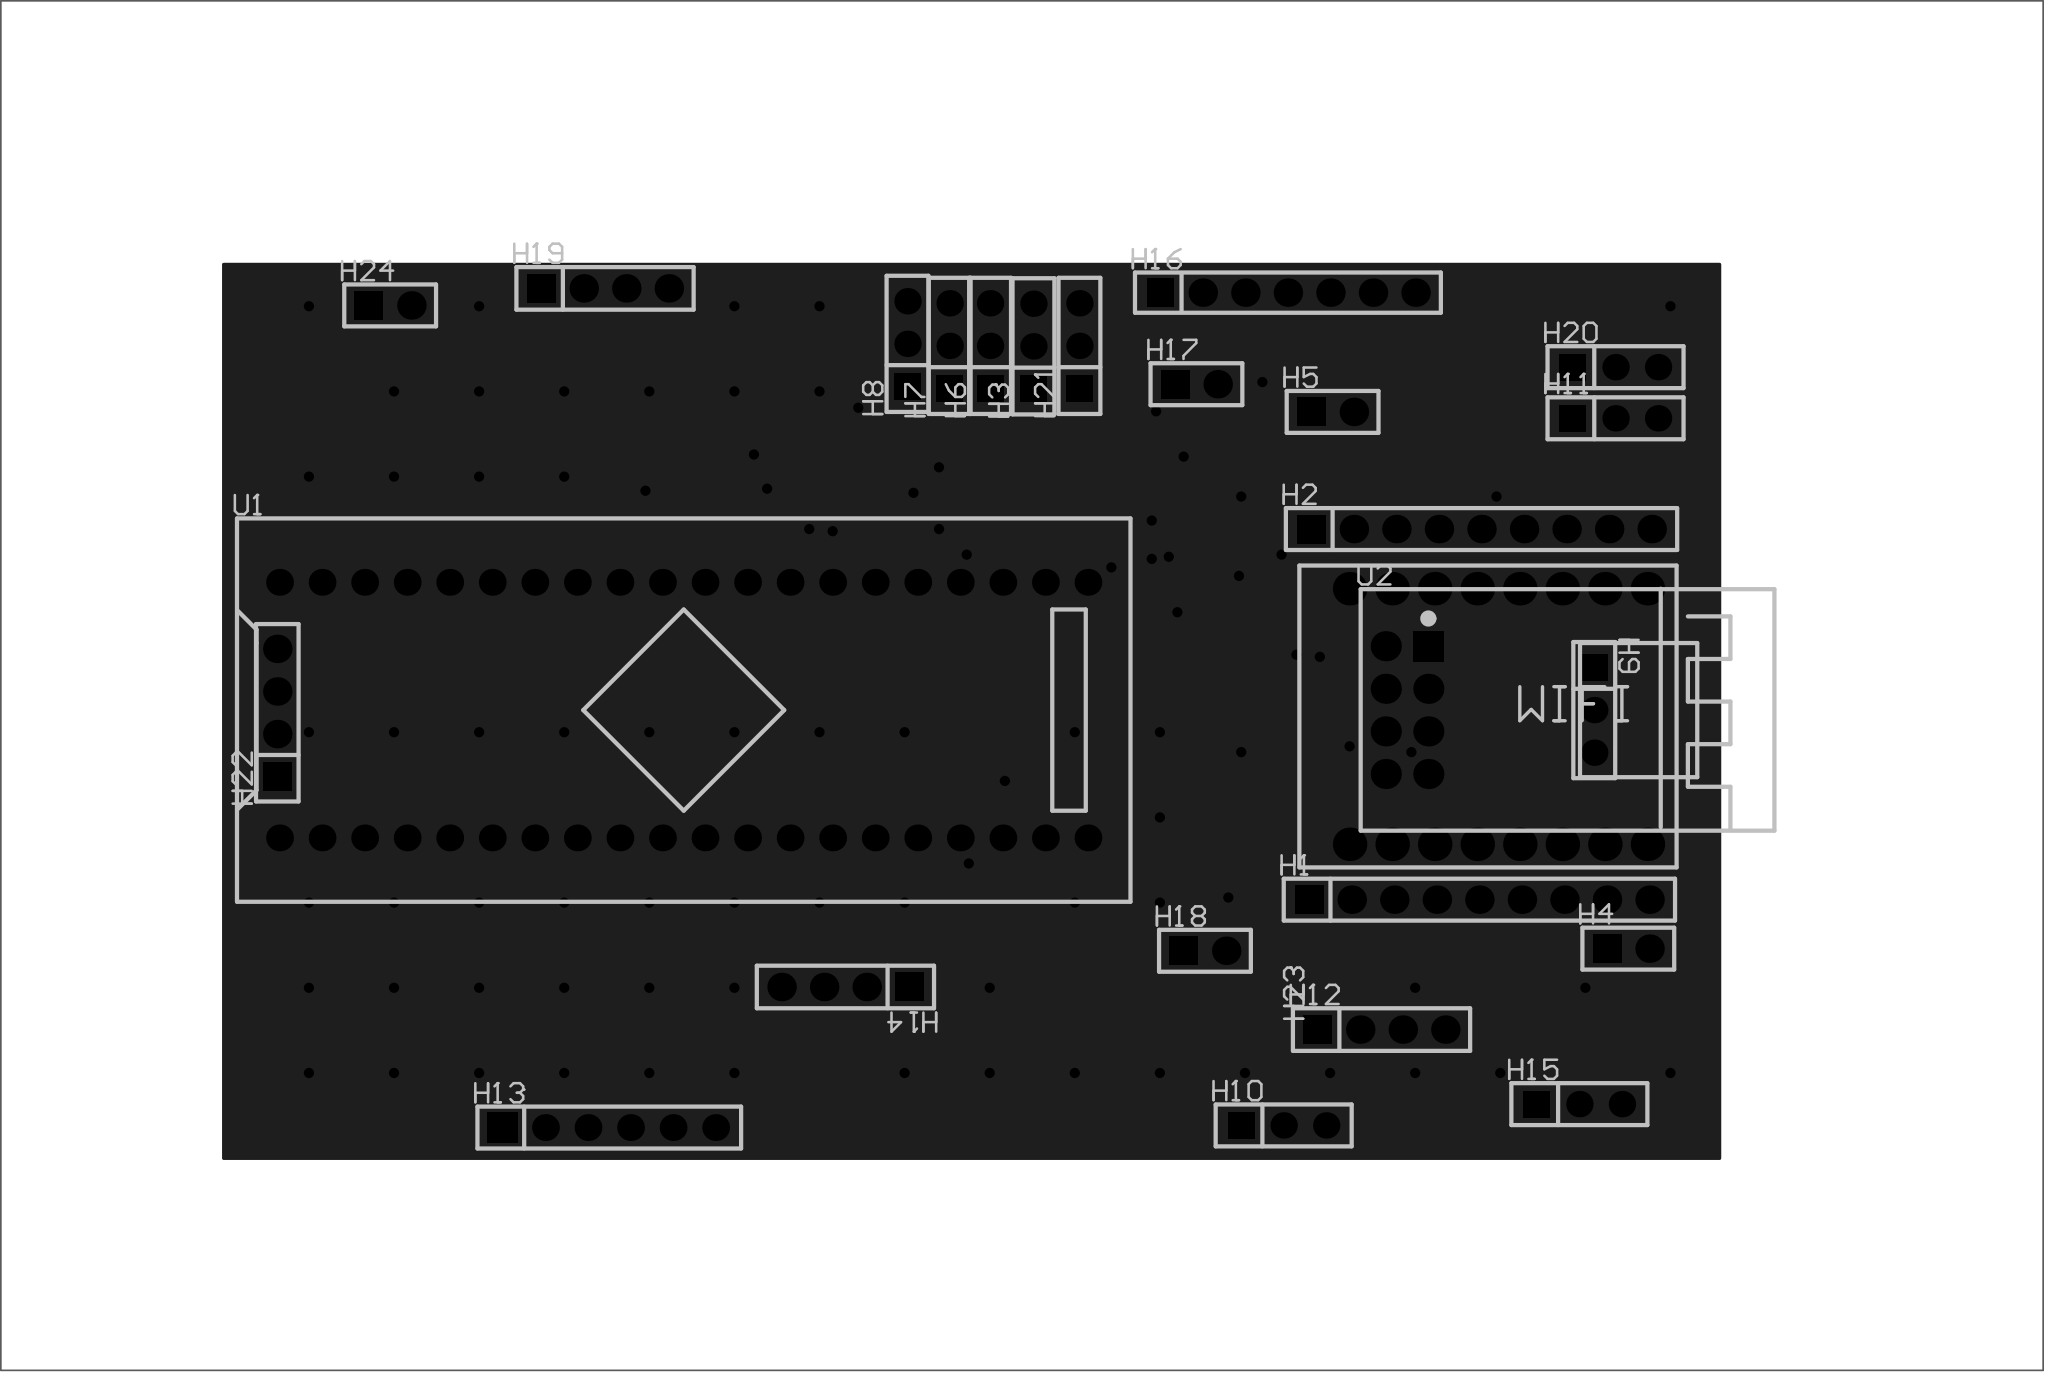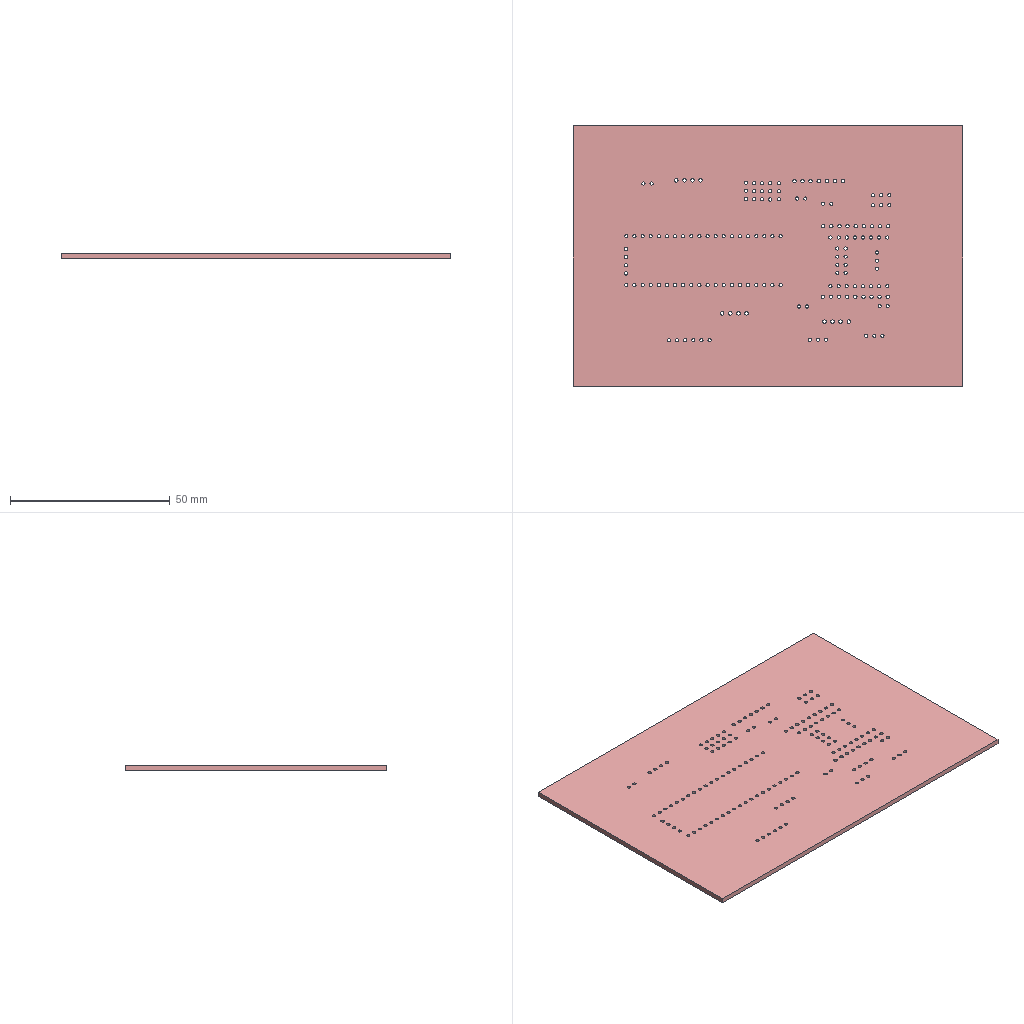Circuit board layout | Altium Designer | box 121.9 x 81.7 x 1.6 mm
Layer stack:
# Altium Designer layer stack of  (unit mm; dielectric type: 0 none, 1 core, 2 prepreg, 3 surface material)
index,name,kind,layer,copper_thickness_mm,dielectric_type,dielectric_thickness_mm,dielectric_material,dielectric_constant
0,Top Paste Mask Layer,other,,,,,,
1,Top Silkscreen Layer,other,,,,,,
2,Top Solder Mask Layer,dielectric,,,3,0.01,,3.3
3,Top Layer,copper,Top Layer,0.035,,,,
4,Dielectric1,dielectric,,,3,1.51,FR4,4.5
5,Bottom Layer,copper,Bottom Layer,0.035,,,,
6,Bottom Solder Mask Layer,dielectric,,,3,0.01,,3.3
7,Bottom Silkscreen Layer,other,,,,,,
8,Bottom Paste Mask Layer,other,,,,,,
# drill layer pairs: low layer,high layer
drill_pair,Top Layer,Bottom Layer
Part placement:
Designator,Comment,Layer,Footprint,Center-X(mm),Center-Y(mm),Rotation
H22,,TopLayer,HDR-TH_4P-P2.54-V-F,86.353,109.06,90
U1,STM32F103C8T6-Card,TopLayer,CONN-TH_L53.3-W22.9_STM32F103C8T6-CARD,110.617,109.22,0
H13,,TopLayer,HDR-TH_6P-P2.54-V-F,106.172,84.328,0
H19,,TopLayer,HDR-TH_4P-P2.54-V-F,105.918,134.366,0
H14,,TopLayer,HDR-TH_4P-P2.54-V-F,120.269,92.71,180
H8,,TopLayer,HDR-TH_3P-P2.54-V-F,123.976,131.058,90
H7,,TopLayer,HDR-TH_3P-P2.54-V-F,126.492,130.937,90
H6,,TopLayer,HDR-TH_3P-P2.54-V-F,128.905,130.937,90
H3,,TopLayer,HDR-TH_3P-P2.54-V-F,131.494,130.91,90
H21,,TopLayer,HDR-TH_3P-P2.54-V-F,134.239,130.937,90
H16,,TopLayer,HDR-TH_7P-P2.54-V-F,146.685,134.112,0
H17,,TopLayer,HDR-TH_2P-P2.54-V-F,141.224,128.651,0
H18,,TopLayer,HDR-TH_2P-P2.54-V-F,141.732,94.869,0
H10,,TopLayer,HDR-TH_3P-P2.54-V-F,146.431,84.455,0
H2,,TopLayer,HDR-TH_9P-P2.54-V-F-1,158.242,120.015,0
H1,,TopLayer,HDR-TH_9P-P2.54-V-F-1,158.115,97.917,0
H5,,TopLayer,HDR-TH_2P-P2.54-V-F,149.352,127,0
H12,,TopLayer,HDR-TH_4P-P2.54-V-F,152.273,90.17,0
U2,Ai-Thinker ESP-01S ESP8266,TopLayer,WIFIM-TH_8P-L24.7-W14.4-P2.54,153.797,109.22,0
H15,,TopLayer,HDR-TH_3P-P2.54-V-F,164.084,85.725,0
H20,,TopLayer,HDR-TH_3P-P2.54-V-F,166.243,129.667,0
H11,,TopLayer,HDR-TH_3P-P2.54-V-F,166.243,126.619,0
H9,,TopLayer,HDR-TH_3P-P2.54-V-F,164.973,109.22,270
H4,,TopLayer,HDR-TH_2P-P2.54-V-F,167.005,94.996,0
H24,,TopLayer,HDR-TH_2P-P2.54-V-F,93.091,133.35,0
H23,,TopLayer,ESP32C3MINI,159.258,108.839,90
Pad and via stacks:
# Altium Designer via and pad stacks of  (unit mm). Each distinct definition once, with the count of objects using it.
# via: kind,start_layer,end_layer,hole_mm,diameter_mm,mode(0 simple;1 top-mid-bottom;2 full stack),diameter_per_layer,count,example_net
# pad: kind,layer,hole_mm,hole_type(0 round;1 square;2 slot),plating,top_size,top_shape(1 round;2 rect;3 octagon;9 rounded rect),mid_size,bottom_size,mode,footprint,size_per_layer,count,example
pad,Multi-Layer,1.1,0,plated,1.7x1.7,2,1.7x1.7,1.7x1.7,0,HDR-TH_4P-P2.54-V-F,,4,H22.1
pad,Multi-Layer,1.1,0,plated,1.7x1.7,1,1.7x1.7,1.7x1.7,0,HDR-TH_4P-P2.54-V-F,,12,H22.2
pad,Multi-Layer,1,0,plated,1.6x1.6,1,1.6x1.6,1.6x1.6,0,CONN-TH_L53.3-W22.9_STM32F103C8T6-CARD,,40,U1.1
pad,Multi-Layer,1.02,0,plated,1.6x1.6,1,1.6x1.6,1.6x1.6,0,HDR-TH_6P-P2.54-V-F,,5,H13.6
pad,Multi-Layer,1.02,0,plated,1.8x1.8,2,1.8x1.8,1.8x1.8,0,HDR-TH_6P-P2.54-V-F,,1,H13.1
pad,Multi-Layer,1.02,0,plated,1.575x1.575,1,1.575x1.575,1.575x1.575,0,HDR-TH_3P-P2.54-V-F,,20,H8.3
pad,Multi-Layer,1.02,0,plated,1.575x1.575,2,1.575x1.575,1.575x1.575,0,HDR-TH_3P-P2.54-V-F,,10,H8.1
pad,Multi-Layer,1.1,0,plated,1.7x1.7,1,1.7x1.7,1.7x1.7,0,HDR-TH_7P-P2.54-V-F,,6,H16.7
pad,Multi-Layer,1.1,0,plated,1.575x1.7,2,1.575x1.7,1.575x1.7,0,HDR-TH_7P-P2.54-V-F,,1,H16.1
pad,Multi-Layer,1,0,plated,1.7x1.7,2,1.7x1.7,1.7x1.7,0,HDR-TH_2P-P2.54-V-F,,5,H17.1
pad,Multi-Layer,1,0,plated,1.7x1.7,1,1.7x1.7,1.7x1.7,0,HDR-TH_2P-P2.54-V-F,,5,H17.2
pad,Multi-Layer,1.1,0,plated,1.7x1.7,2,1.7x1.7,1.7x1.7,0,HDR-TH_9P-P2.54-V-F-1,,2,H2.1
pad,Multi-Layer,1.1,0,plated,1.7x1.7,1,1.7x1.7,1.7x1.7,0,HDR-TH_9P-P2.54-V-F-1,,16,H2.2
pad,Multi-Layer,1,0,plated,1.8x1.8,1,1.8x1.8,1.8x1.8,0,WIFIM-TH_8P-L24.7-W14.4-P2.54,,7,U2.8
pad,Multi-Layer,1,0,plated,1.8x1.8,2,1.8x1.8,1.8x1.8,0,WIFIM-TH_8P-L24.7-W14.4-P2.54,,1,U2.1
pad,Multi-Layer,1,0,plated,2x2,1,2x2,2x2,0,ESP32C3MINI,,16,H23.1
via,Top Layer,Bottom Layer,0.3048,0.61,0,,90,PB8
Copper pours:
name,layer,net,type(0 solid;1 hatched;2 none)
Top Layer-GND,Top Layer,GND,0
Bottom Layer-GND,Bottom Layer,GND,0
Design rules, without the lines most boards share:
# Altium Designer design rules of  (exported by Altium Designer, unit mm)
# columns: name | kind | enabled | priority | scope1 | scope2 | descriptor | typed fields (field=value)
copperThickness1oz_2 | 2 | enabled | 2 | All | All | Width Constraint (Min=30mil) (Max=100mil) (Preferred=30mil) (All) |